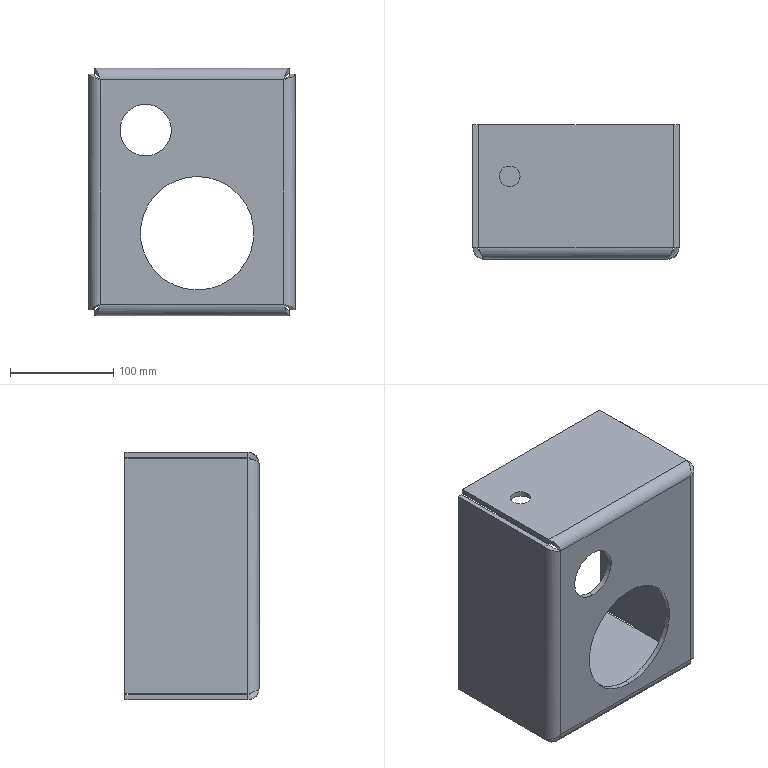Part | SolidWorks | features ICE 5, Cut 1, EdgeFlange 1, FlatPattern 1, SMBaseFlange 1, SheetMetal 1, UnFold 1 | 1 solid | 46 faces | box 200 x 130 x 240 mm | volume 676018 mm3 | plane 22 | cylinder 16 | spline 8 | commonest cylinder face diameters 12 x4 22 x4 50 x4 20 x2 110 x2